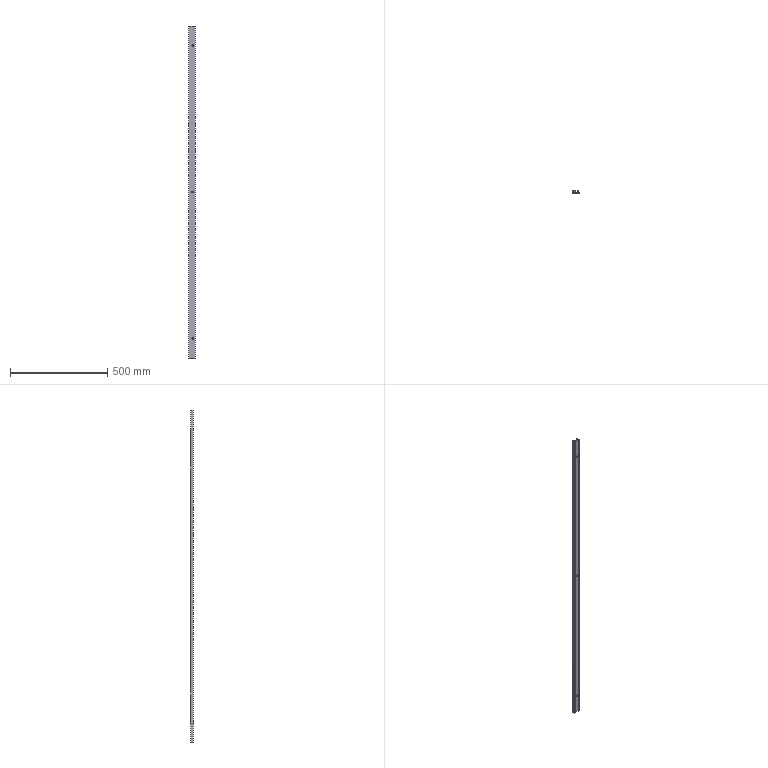Part | SolidWorks | features BaseBody 1, HoleWzd 1, ICE 1, MoveFace 1 | 1 solid | 31 faces | box 33.5 x 13.5 x 1705 mm | volume 319217 mm3 | plane 16 | cylinder 9 | cone 6 | commonest cylinder face diameters 2 x3 13.44 x3 4 x2 1.5 x1
STEP:
#1=CARTESIAN_POINT('',(20.,0.,1508.72));
#2=VERTEX_POINT('',#1);
#3=CARTESIAN_POINT('',(20.,0.,1501.28));
#4=VERTEX_POINT('',#3);
#5=CARTESIAN_POINT('',(20.,0.,1505.));
#6=DIRECTION('',(0.,-1.,0.));
#7=DIRECTION('',(0.,0.,-1.));
#8=AXIS2_PLACEMENT_3D('',#5,#6,#7);
#9=CIRCLE('',#8,3.72);
#10=EDGE_CURVE('',#2,#4,#9,.T.);
#11=ORIENTED_EDGE('',*,*,#10,.T.);
#12=CARTESIAN_POINT('',(20.,3.,1498.28));
#13=VERTEX_POINT('',#12);
#14=CARTESIAN_POINT('',(20.,3.,1498.28));
#15=DIRECTION('',(0.,0.7071,-0.7071));
#16=VECTOR('',#15,1000.);
#17=LINE('',#14,#16);
#18=EDGE_CURVE('',#4,#13,#17,.T.);
#19=ORIENTED_EDGE('',*,*,#18,.T.);
#20=CARTESIAN_POINT('',(20.,3.,1511.72));
#21=VERTEX_POINT('',#20);
#22=CARTESIAN_POINT('',(20.,3.,1505.));
#23=DIRECTION('',(0.,1.,0.));
#24=DIRECTION('',(0.,0.,1.));
#25=AXIS2_PLACEMENT_3D('',#22,#23,#24);
#26=CIRCLE('',#25,6.72);
#27=EDGE_CURVE('',#13,#21,#26,.T.);
#28=ORIENTED_EDGE('',*,*,#27,.T.);
#29=CARTESIAN_POINT('',(20.,3.,1511.72));
#30=DIRECTION('',(0.,0.7071,0.7071));
#31=VECTOR('',#30,1000.);
#32=LINE('',#29,#31);
#33=EDGE_CURVE('',#2,#21,#32,.T.);
#34=ORIENTED_EDGE('',*,*,#33,.F.);
#35=EDGE_LOOP('',(#11,#19,#28,#34));
#36=FACE_OUTER_BOUND('',#35,.T.);
#37=CARTESIAN_POINT('',(20.,3.,1505.));
#38=DIRECTION('',(0.,1.,0.));
#39=DIRECTION('',(0.,0.,1.));
#40=AXIS2_PLACEMENT_3D('',#37,#38,#39);
#41=CONICAL_SURFACE('',#40,6.72,0.7854);
#42=ADVANCED_FACE('',(#36),#41,.F.);
#43=CARTESIAN_POINT('',(20.,0.,3.72));
#44=VERTEX_POINT('',#43);
#45=CARTESIAN_POINT('',(20.,0.,-3.72));
#46=VERTEX_POINT('',#45);
#47=CARTESIAN_POINT('',(20.,0.,0.));
#48=DIRECTION('',(0.,-1.,0.));
#49=DIRECTION('',(0.,0.,-1.));
#50=AXIS2_PLACEMENT_3D('',#47,#48,#49);
#51=CIRCLE('',#50,3.72);
#52=EDGE_CURVE('',#44,#46,#51,.T.);
#53=ORIENTED_EDGE('',*,*,#52,.T.);
#54=CARTESIAN_POINT('',(20.,3.,-6.72));
#55=VERTEX_POINT('',#54);
#56=CARTESIAN_POINT('',(20.,3.,-6.72));
#57=DIRECTION('',(0.,0.7071,-0.7071));
#58=VECTOR('',#57,1000.);
#59=LINE('',#56,#58);
#60=EDGE_CURVE('',#46,#55,#59,.T.);
#61=ORIENTED_EDGE('',*,*,#60,.T.);
#62=CARTESIAN_POINT('',(20.,3.,6.72));
#63=VERTEX_POINT('',#62);
#64=CARTESIAN_POINT('',(20.,3.,0.));
#65=DIRECTION('',(0.,1.,0.));
#66=DIRECTION('',(0.,0.,1.));
#67=AXIS2_PLACEMENT_3D('',#64,#65,#66);
#68=CIRCLE('',#67,6.72);
#69=EDGE_CURVE('',#55,#63,#68,.T.);
#70=ORIENTED_EDGE('',*,*,#69,.T.);
#71=CARTESIAN_POINT('',(20.,3.,6.72));
#72=DIRECTION('',(0.,0.7071,0.7071));
#73=VECTOR('',#72,1000.);
#74=LINE('',#71,#73);
#75=EDGE_CURVE('',#44,#63,#74,.T.);
#76=ORIENTED_EDGE('',*,*,#75,.F.);
#77=EDGE_LOOP('',(#53,#61,#70,#76));
#78=FACE_OUTER_BOUND('',#77,.T.);
#79=CARTESIAN_POINT('',(20.,3.,0.));
#80=DIRECTION('',(0.,1.,0.));
#81=DIRECTION('',(0.,0.,1.));
#82=AXIS2_PLACEMENT_3D('',#79,#80,#81);
#83=CONICAL_SURFACE('',#82,6.72,0.7854);
#84=ADVANCED_FACE('',(#78),#83,.F.);
#85=CARTESIAN_POINT('',(20.,0.,756.22));
#86=VERTEX_POINT('',#85);
#87=CARTESIAN_POINT('',(20.,0.,748.78));
#88=VERTEX_POINT('',#87);
#89=CARTESIAN_POINT('',(20.,0.,752.5));
#90=DIRECTION('',(0.,-1.,0.));
#91=DIRECTION('',(0.,0.,-1.));
#92=AXIS2_PLACEMENT_3D('',#89,#90,#91);
#93=CIRCLE('',#92,3.72);
#94=EDGE_CURVE('',#86,#88,#93,.T.);
#95=ORIENTED_EDGE('',*,*,#94,.T.);
#96=CARTESIAN_POINT('',(20.,3.,745.78));
#97=VERTEX_POINT('',#96);
#98=CARTESIAN_POINT('',(20.,3.,745.78));
#99=DIRECTION('',(0.,0.7071,-0.7071));
#100=VECTOR('',#99,1000.);
#101=LINE('',#98,#100);
#102=EDGE_CURVE('',#88,#97,#101,.T.);
#103=ORIENTED_EDGE('',*,*,#102,.T.);
#104=CARTESIAN_POINT('',(20.,3.,759.22));
#105=VERTEX_POINT('',#104);
#106=CARTESIAN_POINT('',(20.,3.,752.5));
#107=DIRECTION('',(0.,1.,0.));
#108=DIRECTION('',(0.,0.,1.));
#109=AXIS2_PLACEMENT_3D('',#106,#107,#108);
#110=CIRCLE('',#109,6.72);
#111=EDGE_CURVE('',#97,#105,#110,.T.);
#112=ORIENTED_EDGE('',*,*,#111,.T.);
#113=CARTESIAN_POINT('',(20.,3.,759.22));
#114=DIRECTION('',(0.,0.7071,0.7071));
#115=VECTOR('',#114,1000.);
#116=LINE('',#113,#115);
#117=EDGE_CURVE('',#86,#105,#116,.T.);
#118=ORIENTED_EDGE('',*,*,#117,.F.);
#119=EDGE_LOOP('',(#95,#103,#112,#118));
#120=FACE_OUTER_BOUND('',#119,.T.);
#121=CARTESIAN_POINT('',(20.,3.,752.5));
#122=DIRECTION('',(0.,1.,0.));
#123=DIRECTION('',(0.,0.,1.));
#124=AXIS2_PLACEMENT_3D('',#121,#122,#123);
#125=CONICAL_SURFACE('',#124,6.72,0.7854);
#126=ADVANCED_FACE('',(#120),#125,.F.);
#127=CARTESIAN_POINT('',(24.5,10.5,-4.991));
#128=VERTEX_POINT('',#127);
#129=CARTESIAN_POINT('',(24.5,10.5,-100.));
#130=VERTEX_POINT('',#129);
#131=CARTESIAN_POINT('',(24.5,10.5,-100.));
#132=DIRECTION('',(0.,0.,-1.));
#133=VECTOR('',#132,1000.);
#134=LINE('',#131,#133);
#135=EDGE_CURVE('',#128,#130,#134,.T.);
#136=ORIENTED_EDGE('',*,*,#135,.F.);
#137=CARTESIAN_POINT('',(24.5,10.5,4.991));
#138=VERTEX_POINT('',#137);
#139=CARTESIAN_POINT('',(24.5,10.5,-4.991));
#140=CARTESIAN_POINT('',(24.5,10.638,-4.991));
#141=CARTESIAN_POINT('',(24.515,10.777,-4.978));
#142=CARTESIAN_POINT('',(24.57,11.043,-4.927));
#143=CARTESIAN_POINT('',(24.611,11.171,-4.889));
#144=CARTESIAN_POINT('',(24.765,11.529,-4.74));
#145=CARTESIAN_POINT('',(24.907,11.728,-4.597));
#146=CARTESIAN_POINT('',(25.205,12.04,-4.256));
#147=CARTESIAN_POINT('',(25.365,12.156,-4.055));
#148=CARTESIAN_POINT('',(25.663,12.325,-3.627));
#149=CARTESIAN_POINT('',(25.806,12.38,-3.395));
#150=CARTESIAN_POINT('',(26.19,12.494,-2.672));
#151=CARTESIAN_POINT('',(26.387,12.501,-2.161));
#152=CARTESIAN_POINT('',(26.654,12.499,-1.091));
#153=CARTESIAN_POINT('',(26.72,12.488,-0.5481));
#154=CARTESIAN_POINT('',(26.72,12.488,0.2773));
#155=CARTESIAN_POINT('',(26.703,12.49,0.5529));
#156=CARTESIAN_POINT('',(26.636,12.496,1.095));
#157=CARTESIAN_POINT('',(26.586,12.499,1.362));
#158=CARTESIAN_POINT('',(26.388,12.501,2.155));
#159=CARTESIAN_POINT('',(26.188,12.493,2.677));
#160=CARTESIAN_POINT('',(25.805,12.38,3.396));
#161=CARTESIAN_POINT('',(25.662,12.324,3.629));
#162=CARTESIAN_POINT('',(25.438,12.197,3.95));
#163=CARTESIAN_POINT('',(25.362,12.147,4.053));
#164=CARTESIAN_POINT('',(25.208,12.03,4.249));
#165=CARTESIAN_POINT('',(25.13,11.961,4.342));
#166=CARTESIAN_POINT('',(24.98,11.805,4.513));
#167=CARTESIAN_POINT('',(24.908,11.717,4.591));
#168=CARTESIAN_POINT('',(24.774,11.518,4.73));
#169=CARTESIAN_POINT('',(24.714,11.408,4.79));
#170=CARTESIAN_POINT('',(24.612,11.172,4.888));
#171=CARTESIAN_POINT('',(24.57,11.043,4.927));
#172=CARTESIAN_POINT('',(24.515,10.778,4.978));
#173=CARTESIAN_POINT('',(24.5,10.64,4.991));
#174=CARTESIAN_POINT('',(24.5,10.5,4.991));
#175=B_SPLINE_CURVE_WITH_KNOTS('',3,(#139,#140,#141,#142,#143,#144,#145,#146,#147,#148,#149,#150,#151,#152,#153,#154,#155,#156,#157,#158,#159,#160,#161,#162,#163,#164,#165,#166,#167,#168,#169,#170,#171,#172,#173,#174),.UNSPECIFIED.,.F.,.F.,(4,2,2,2,2,2,2,2,2,2,2,2,2,2,2,2,2,4),(0.01321,0.01362,0.01403,0.01486,0.01569,0.01651,0.01816,0.01981,0.02064,0.02146,0.02311,0.02394,0.02435,0.02477,0.02518,0.02559,0.026,0.02642),.UNSPECIFIED.);
#176=EDGE_CURVE('',#128,#138,#175,.T.);
#177=ORIENTED_EDGE('',*,*,#176,.T.);
#178=CARTESIAN_POINT('',(24.5,10.5,747.509));
#179=VERTEX_POINT('',#178);
#180=CARTESIAN_POINT('',(24.5,10.5,-100.));
#181=DIRECTION('',(0.,0.,-1.));
#182=VECTOR('',#181,1000.);
#183=LINE('',#180,#182);
#184=EDGE_CURVE('',#179,#138,#183,.T.);
#185=ORIENTED_EDGE('',*,*,#184,.F.);
#186=CARTESIAN_POINT('',(24.5,10.5,757.491));
#187=VERTEX_POINT('',#186);
#188=CARTESIAN_POINT('',(24.5,10.5,747.509));
#189=CARTESIAN_POINT('',(24.5,10.638,747.509));
#190=CARTESIAN_POINT('',(24.515,10.777,747.522));
#191=CARTESIAN_POINT('',(24.57,11.043,747.573));
#192=CARTESIAN_POINT('',(24.611,11.171,747.611));
#193=CARTESIAN_POINT('',(24.765,11.529,747.76));
#194=CARTESIAN_POINT('',(24.907,11.728,747.903));
#195=CARTESIAN_POINT('',(25.205,12.04,748.244));
#196=CARTESIAN_POINT('',(25.365,12.156,748.445));
#197=CARTESIAN_POINT('',(25.663,12.325,748.873));
#198=CARTESIAN_POINT('',(25.806,12.38,749.105));
#199=CARTESIAN_POINT('',(26.19,12.494,749.828));
#200=CARTESIAN_POINT('',(26.387,12.501,750.339));
#201=CARTESIAN_POINT('',(26.654,12.499,751.409));
#202=CARTESIAN_POINT('',(26.72,12.488,751.952));
#203=CARTESIAN_POINT('',(26.72,12.488,752.777));
#204=CARTESIAN_POINT('',(26.703,12.49,753.053));
#205=CARTESIAN_POINT('',(26.636,12.496,753.595));
#206=CARTESIAN_POINT('',(26.586,12.499,753.862));
#207=CARTESIAN_POINT('',(26.388,12.501,754.655));
#208=CARTESIAN_POINT('',(26.188,12.493,755.177));
#209=CARTESIAN_POINT('',(25.805,12.38,755.896));
#210=CARTESIAN_POINT('',(25.662,12.324,756.129));
#211=CARTESIAN_POINT('',(25.438,12.197,756.45));
#212=CARTESIAN_POINT('',(25.362,12.147,756.553));
#213=CARTESIAN_POINT('',(25.208,12.03,756.749));
#214=CARTESIAN_POINT('',(25.13,11.961,756.842));
#215=CARTESIAN_POINT('',(24.98,11.805,757.013));
#216=CARTESIAN_POINT('',(24.908,11.717,757.091));
#217=CARTESIAN_POINT('',(24.774,11.518,757.23));
#218=CARTESIAN_POINT('',(24.714,11.408,757.29));
#219=CARTESIAN_POINT('',(24.612,11.172,757.388));
#220=CARTESIAN_POINT('',(24.57,11.043,757.427));
#221=CARTESIAN_POINT('',(24.515,10.778,757.478));
#222=CARTESIAN_POINT('',(24.5,10.64,757.491));
#223=CARTESIAN_POINT('',(24.5,10.5,757.491));
#224=B_SPLINE_CURVE_WITH_KNOTS('',3,(#188,#189,#190,#191,#192,#193,#194,#195,#196,#197,#198,#199,#200,#201,#202,#203,#204,#205,#206,#207,#208,#209,#210,#211,#212,#213,#214,#215,#216,#217,#218,#219,#220,#221,#222,#223),.UNSPECIFIED.,.F.,.F.,(4,2,2,2,2,2,2,2,2,2,2,2,2,2,2,2,2,4),(0.01321,0.01362,0.01403,0.01486,0.01569,0.01651,0.01816,0.01981,0.02064,0.02146,0.02311,0.02394,0.02435,0.02477,0.02518,0.02559,0.026,0.02642),.UNSPECIFIED.);
#225=EDGE_CURVE('',#179,#187,#224,.T.);
#226=ORIENTED_EDGE('',*,*,#225,.T.);
#227=CARTESIAN_POINT('',(24.5,10.5,1500.009));
#228=VERTEX_POINT('',#227);
#229=CARTESIAN_POINT('',(24.5,10.5,-100.));
#230=DIRECTION('',(0.,0.,-1.));
#231=VECTOR('',#230,1000.);
#232=LINE('',#229,#231);
#233=EDGE_CURVE('',#228,#187,#232,.T.);
#234=ORIENTED_EDGE('',*,*,#233,.F.);
#235=CARTESIAN_POINT('',(24.5,10.5,1509.991));
#236=VERTEX_POINT('',#235);
#237=CARTESIAN_POINT('',(24.5,10.5,1500.009));
#238=CARTESIAN_POINT('',(24.5,10.64,1500.009));
#239=CARTESIAN_POINT('',(24.514,10.776,1500.022));
#240=CARTESIAN_POINT('',(24.57,11.042,1500.073));
#241=CARTESIAN_POINT('',(24.611,11.171,1500.111));
#242=CARTESIAN_POINT('',(24.713,11.408,1500.209));
#243=CARTESIAN_POINT('',(24.775,11.519,1500.27));
#244=CARTESIAN_POINT('',(24.908,11.717,1500.409));
#245=CARTESIAN_POINT('',(24.981,11.806,1500.488));
#246=CARTESIAN_POINT('',(25.207,12.042,1500.746));
#247=CARTESIAN_POINT('',(25.363,12.155,1500.942));
#248=CARTESIAN_POINT('',(25.665,12.326,1501.376));
#249=CARTESIAN_POINT('',(25.806,12.38,1501.605));
#250=CARTESIAN_POINT('',(26.061,12.456,1502.084));
#251=CARTESIAN_POINT('',(26.176,12.476,1502.337));
#252=CARTESIAN_POINT('',(26.372,12.498,1502.849));
#253=CARTESIAN_POINT('',(26.454,12.501,1503.109));
#254=CARTESIAN_POINT('',(26.586,12.499,1503.638));
#255=CARTESIAN_POINT('',(26.636,12.496,1503.907));
#256=CARTESIAN_POINT('',(26.703,12.49,1504.453));
#257=CARTESIAN_POINT('',(26.72,12.488,1504.729));
#258=CARTESIAN_POINT('',(26.72,12.488,1505.275));
#259=CARTESIAN_POINT('',(26.703,12.49,1505.547));
#260=CARTESIAN_POINT('',(26.637,12.496,1506.089));
#261=CARTESIAN_POINT('',(26.587,12.499,1506.36));
#262=CARTESIAN_POINT('',(26.387,12.501,1507.161));
#263=CARTESIAN_POINT('',(26.191,12.494,1507.671));
#264=CARTESIAN_POINT('',(25.805,12.38,1508.396));
#265=CARTESIAN_POINT('',(25.663,12.325,1508.627));
#266=CARTESIAN_POINT('',(25.364,12.155,1509.057));
#267=CARTESIAN_POINT('',(25.205,12.039,1509.256));
#268=CARTESIAN_POINT('',(24.981,11.805,1509.512));
#269=CARTESIAN_POINT('',(24.907,11.716,1509.592));
#270=CARTESIAN_POINT('',(24.774,11.518,1509.73));
#271=CARTESIAN_POINT('',(24.714,11.409,1509.79));
#272=CARTESIAN_POINT('',(24.611,11.17,1509.889));
#273=CARTESIAN_POINT('',(24.571,11.044,1509.926));
#274=CARTESIAN_POINT('',(24.515,10.78,1509.977));
#275=CARTESIAN_POINT('',(24.5,10.64,1509.991));
#276=CARTESIAN_POINT('',(24.5,10.5,1509.991));
#277=B_SPLINE_CURVE_WITH_KNOTS('',3,(#237,#238,#239,#240,#241,#242,#243,#244,#245,#246,#247,#248,#249,#250,#251,#252,#253,#254,#255,#256,#257,#258,#259,#260,#261,#262,#263,#264,#265,#266,#267,#268,#269,#270,#271,#272,#273,#274,#275,#276),.UNSPECIFIED.,.F.,.F.,(4,2,2,2,2,2,2,2,2,2,2,2,2,2,2,2,2,2,2,4),(0.,0.0004127,0.0008255,0.001238,0.001651,0.002476,0.003302,0.004127,0.004953,0.005778,0.006604,0.007429,0.008255,0.009906,0.01073,0.01156,0.01197,0.01238,0.01279,0.01321),.UNSPECIFIED.);
#278=EDGE_CURVE('',#228,#236,#277,.T.);
#279=ORIENTED_EDGE('',*,*,#278,.T.);
#280=CARTESIAN_POINT('',(24.5,10.5,1605.));
#281=VERTEX_POINT('',#280);
#282=CARTESIAN_POINT('',(24.5,10.5,-100.));
#283=DIRECTION('',(0.,0.,-1.));
#284=VECTOR('',#283,1000.);
#285=LINE('',#282,#284);
#286=EDGE_CURVE('',#281,#236,#285,.T.);
#287=ORIENTED_EDGE('',*,*,#286,.F.);
#288=CARTESIAN_POINT('',(28.5,10.5,1605.));
#289=VERTEX_POINT('',#288);
#290=CARTESIAN_POINT('',(26.5,10.5,1605.));
#291=DIRECTION('',(0.,0.,1.));
#292=DIRECTION('',(1.,0.,0.));
#293=AXIS2_PLACEMENT_3D('',#290,#291,#292);
#294=CIRCLE('',#293,2.);
#295=EDGE_CURVE('',#289,#281,#294,.T.);
#296=ORIENTED_EDGE('',*,*,#295,.F.);
#297=CARTESIAN_POINT('',(28.5,10.5,-100.));
#298=VERTEX_POINT('',#297);
#299=CARTESIAN_POINT('',(28.5,10.5,-100.));
#300=DIRECTION('',(0.,0.,-1.));
#301=VECTOR('',#300,1000.);
#302=LINE('',#299,#301);
#303=EDGE_CURVE('',#289,#298,#302,.T.);
#304=ORIENTED_EDGE('',*,*,#303,.T.);
#305=CARTESIAN_POINT('',(26.5,10.5,-100.));
#306=DIRECTION('',(0.,0.,1.));
#307=DIRECTION('',(-1.,0.,0.));
#308=AXIS2_PLACEMENT_3D('',#305,#306,#307);
#309=CIRCLE('',#308,2.);
#310=EDGE_CURVE('',#298,#130,#309,.T.);
#311=ORIENTED_EDGE('',*,*,#310,.T.);
#312=EDGE_LOOP('',(#136,#177,#185,#226,#234,#279,#287,#296,#304,#311));
#313=FACE_OUTER_BOUND('',#312,.T.);
#314=CARTESIAN_POINT('',(26.5,10.5,-100.));
#315=DIRECTION('',(0.,0.,-1.));
#316=DIRECTION('',(-1.,0.,0.));
#317=AXIS2_PLACEMENT_3D('',#314,#315,#316);
#318=CYLINDRICAL_SURFACE('',#317,2.);
#319=ADVANCED_FACE('',(#313),#318,.T.);
#320=CARTESIAN_POINT('',(24.5,3.,-4.991));
#321=VERTEX_POINT('',#320);
#322=CARTESIAN_POINT('',(24.5,3.,-100.));
#323=VERTEX_POINT('',#322);
#324=CARTESIAN_POINT('',(24.5,3.,-100.));
#325=DIRECTION('',(0.,0.,-1.));
#326=VECTOR('',#325,1000.);
#327=LINE('',#324,#326);
#328=EDGE_CURVE('',#321,#323,#327,.T.);
#329=ORIENTED_EDGE('',*,*,#328,.F.);
#330=CARTESIAN_POINT('',(24.5,13.5,-4.991));
#331=DIRECTION('',(0.,1.,0.));
#332=VECTOR('',#331,1000.);
#333=LINE('',#330,#332);
#334=EDGE_CURVE('',#321,#128,#333,.T.);
#335=ORIENTED_EDGE('',*,*,#334,.T.);
#336=ORIENTED_EDGE('',*,*,#135,.T.);
#337=CARTESIAN_POINT('',(24.5,1.,-100.));
#338=DIRECTION('',(0.,-1.,0.));
#339=VECTOR('',#338,1000.);
#340=LINE('',#337,#339);
#341=EDGE_CURVE('',#130,#323,#340,.T.);
#342=ORIENTED_EDGE('',*,*,#341,.T.);
#343=EDGE_LOOP('',(#329,#335,#336,#342));
#344=FACE_OUTER_BOUND('',#343,.T.);
#345=CARTESIAN_POINT('',(24.5,10.5,-100.));
#346=DIRECTION('',(-1.,0.,0.));
#347=DIRECTION('',(0.,0.,1.));
#348=AXIS2_PLACEMENT_3D('',#345,#346,#347);
#349=PLANE('',#348);
#350=ADVANCED_FACE('',(#344),#349,.T.);
#351=ORIENTED_EDGE('',*,*,#184,.T.);
#352=CARTESIAN_POINT('',(24.5,3.,4.991));
#353=VERTEX_POINT('',#352);
#354=CARTESIAN_POINT('',(24.5,13.5,4.991));
#355=DIRECTION('',(0.,-1.,0.));
#356=VECTOR('',#355,1000.);
#357=LINE('',#354,#356);
#358=EDGE_CURVE('',#138,#353,#357,.T.);
#359=ORIENTED_EDGE('',*,*,#358,.T.);
#360=CARTESIAN_POINT('',(24.5,3.,747.509));
#361=VERTEX_POINT('',#360);
#362=CARTESIAN_POINT('',(24.5,3.,-100.));
#363=DIRECTION('',(0.,0.,-1.));
#364=VECTOR('',#363,1000.);
#365=LINE('',#362,#364);
#366=EDGE_CURVE('',#361,#353,#365,.T.);
#367=ORIENTED_EDGE('',*,*,#366,.F.);
#368=CARTESIAN_POINT('',(24.5,13.5,747.509));
#369=DIRECTION('',(0.,1.,0.));
#370=VECTOR('',#369,1000.);
#371=LINE('',#368,#370);
#372=EDGE_CURVE('',#361,#179,#371,.T.);
#373=ORIENTED_EDGE('',*,*,#372,.T.);
#374=EDGE_LOOP('',(#351,#359,#367,#373));
#375=FACE_OUTER_BOUND('',#374,.T.);
#376=CARTESIAN_POINT('',(24.5,10.5,-100.));
#377=DIRECTION('',(-1.,0.,0.));
#378=DIRECTION('',(0.,0.,1.));
#379=AXIS2_PLACEMENT_3D('',#376,#377,#378);
#380=PLANE('',#379);
#381=ADVANCED_FACE('',(#375),#380,.T.);
#382=ORIENTED_EDGE('',*,*,#233,.T.);
#383=CARTESIAN_POINT('',(24.5,3.,757.491));
#384=VERTEX_POINT('',#383);
#385=CARTESIAN_POINT('',(24.5,13.5,757.491));
#386=DIRECTION('',(0.,-1.,0.));
#387=VECTOR('',#386,1000.);
#388=LINE('',#385,#387);
#389=EDGE_CURVE('',#187,#384,#388,.T.);
#390=ORIENTED_EDGE('',*,*,#389,.T.);
#391=CARTESIAN_POINT('',(24.5,3.,1500.009));
#392=VERTEX_POINT('',#391);
#393=CARTESIAN_POINT('',(24.5,3.,-100.));
#394=DIRECTION('',(0.,0.,-1.));
#395=VECTOR('',#394,1000.);
#396=LINE('',#393,#395);
#397=EDGE_CURVE('',#392,#384,#396,.T.);
#398=ORIENTED_EDGE('',*,*,#397,.F.);
#399=CARTESIAN_POINT('',(24.5,13.5,1500.009));
#400=DIRECTION('',(0.,1.,0.));
#401=VECTOR('',#400,1000.);
#402=LINE('',#399,#401);
#403=EDGE_CURVE('',#392,#228,#402,.T.);
#404=ORIENTED_EDGE('',*,*,#403,.T.);
#405=EDGE_LOOP('',(#382,#390,#398,#404));
#406=FACE_OUTER_BOUND('',#405,.T.);
#407=CARTESIAN_POINT('',(24.5,10.5,-100.));
#408=DIRECTION('',(-1.,0.,0.));
#409=DIRECTION('',(0.,0.,1.));
#410=AXIS2_PLACEMENT_3D('',#407,#408,#409);
#411=PLANE('',#410);
#412=ADVANCED_FACE('',(#406),#411,.T.);
#413=ORIENTED_EDGE('',*,*,#286,.T.);
#414=CARTESIAN_POINT('',(24.5,3.,1509.991));
#415=VERTEX_POINT('',#414);
#416=CARTESIAN_POINT('',(24.5,13.5,1509.991));
#417=DIRECTION('',(0.,-1.,0.));
#418=VECTOR('',#417,1000.);
#419=LINE('',#416,#418);
#420=EDGE_CURVE('',#236,#415,#419,.T.);
#421=ORIENTED_EDGE('',*,*,#420,.T.);
#422=CARTESIAN_POINT('',(24.5,3.,1605.));
#423=VERTEX_POINT('',#422);
#424=CARTESIAN_POINT('',(24.5,3.,-100.));
#425=DIRECTION('',(0.,0.,-1.));
#426=VECTOR('',#425,1000.);
#427=LINE('',#424,#426);
#428=EDGE_CURVE('',#423,#415,#427,.T.);
#429=ORIENTED_EDGE('',*,*,#428,.F.);
#430=CARTESIAN_POINT('',(24.5,1.,1605.));
#431=DIRECTION('',(0.,-1.,0.));
#432=VECTOR('',#431,1000.);
#433=LINE('',#430,#432);
#434=EDGE_CURVE('',#281,#423,#433,.T.);
#435=ORIENTED_EDGE('',*,*,#434,.F.);
#436=EDGE_LOOP('',(#413,#421,#429,#435));
#437=FACE_OUTER_BOUND('',#436,.T.);
#438=CARTESIAN_POINT('',(24.5,10.5,-100.));
#439=DIRECTION('',(-1.,0.,0.));
#440=DIRECTION('',(0.,0.,1.));
#441=AXIS2_PLACEMENT_3D('',#438,#439,#440);
#442=PLANE('',#441);
#443=ADVANCED_FACE('',(#437),#442,.T.);
#444=ORIENTED_EDGE('',*,*,#10,.F.);
#445=CARTESIAN_POINT('',(20.,0.,1505.));
#446=DIRECTION('',(0.,-1.,0.));
#447=DIRECTION('',(0.,0.,-1.));
#448=AXIS2_PLACEMENT_3D('',#445,#446,#447);
#449=CIRCLE('',#448,3.72);
#450=EDGE_CURVE('',#4,#2,#449,.T.);
#451=ORIENTED_EDGE('',*,*,#450,.F.);
#452=EDGE_LOOP('',(#444,#451));
#453=FACE_BOUND('',#452,.T.);
#454=ORIENTED_EDGE('',*,*,#94,.F.);
#455=CARTESIAN_POINT('',(20.,0.,752.5));
#456=DIRECTION('',(0.,-1.,0.));
#457=DIRECTION('',(0.,0.,-1.));
#458=AXIS2_PLACEMENT_3D('',#455,#456,#457);
#459=CIRCLE('',#458,3.72);
#460=EDGE_CURVE('',#88,#86,#459,.T.);
#461=ORIENTED_EDGE('',*,*,#460,.F.);
#462=EDGE_LOOP('',(#454,#461));
#463=FACE_BOUND('',#462,.T.);
#464=CARTESIAN_POINT('',(1.,0.,-100.));
#465=VERTEX_POINT('',#464);
#466=CARTESIAN_POINT('',(32.5,0.,-100.));
#467=VERTEX_POINT('',#466);
#468=CARTESIAN_POINT('',(1.,0.,-100.));
#469=DIRECTION('',(1.,0.,0.));
#470=VECTOR('',#469,1000.);
#471=LINE('',#468,#470);
#472=EDGE_CURVE('',#465,#467,#471,.T.);
#473=ORIENTED_EDGE('',*,*,#472,.T.);
#474=CARTESIAN_POINT('',(32.5,0.,1605.));
#475=VERTEX_POINT('',#474);
#476=CARTESIAN_POINT('',(32.5,0.,-100.));
#477=DIRECTION('',(0.,0.,1.));
#478=VECTOR('',#477,1000.);
#479=LINE('',#476,#478);
#480=EDGE_CURVE('',#467,#475,#479,.T.);
#481=ORIENTED_EDGE('',*,*,#480,.T.);
#482=CARTESIAN_POINT('',(1.,0.,1605.));
#483=VERTEX_POINT('',#482);
#484=CARTESIAN_POINT('',(1.,0.,1605.));
#485=DIRECTION('',(-1.,0.,0.));
#486=VECTOR('',#485,1000.);
#487=LINE('',#484,#486);
#488=EDGE_CURVE('',#475,#483,#487,.T.);
#489=ORIENTED_EDGE('',*,*,#488,.T.);
#490=CARTESIAN_POINT('',(1.,0.,-100.));
#491=DIRECTION('',(0.,0.,-1.));
#492=VECTOR('',#491,1000.);
#493=LINE('',#490,#492);
#494=EDGE_CURVE('',#483,#465,#493,.T.);
#495=ORIENTED_EDGE('',*,*,#494,.T.);
#496=EDGE_LOOP('',(#473,#481,#489,#495));
#497=FACE_OUTER_BOUND('',#496,.T.);
#498=ORIENTED_EDGE('',*,*,#52,.F.);
#499=CARTESIAN_POINT('',(20.,0.,0.));
#500=DIRECTION('',(0.,-1.,0.));
#501=DIRECTION('',(0.,0.,-1.));
#502=AXIS2_PLACEMENT_3D('',#499,#500,#501);
#503=CIRCLE('',#502,3.72);
#504=EDGE_CURVE('',#46,#44,#503,.T.);
#505=ORIENTED_EDGE('',*,*,#504,.F.);
#506=EDGE_LOOP('',(#498,#505));
#507=FACE_BOUND('',#506,.T.);
#508=CARTESIAN_POINT('',(1.,0.,-100.));
#509=DIRECTION('',(0.,-1.,0.));
#510=DIRECTION('',(0.,0.,-1.));
#511=AXIS2_PLACEMENT_3D('',#508,#509,#510);
#512=PLANE('',#511);
#513=ADVANCED_FACE('',(#453,#463,#497,#507),#512,.T.);
#514=CARTESIAN_POINT('',(33.5,1.,-100.));
#515=VERTEX_POINT('',#514);
#516=CARTESIAN_POINT('',(32.5,1.,-100.));
#517=DIRECTION('',(0.,0.,1.));
#518=DIRECTION('',(-1.,0.,0.));
#519=AXIS2_PLACEMENT_3D('',#516,#517,#518);
#520=CIRCLE('',#519,1.);
#521=EDGE_CURVE('',#467,#515,#520,.T.);
#522=ORIENTED_EDGE('',*,*,#521,.T.);
#523=CARTESIAN_POINT('',(33.5,1.,1605.));
#524=VERTEX_POINT('',#523);
#525=CARTESIAN_POINT('',(33.5,1.,-100.));
#526=DIRECTION('',(0.,0.,1.));
#527=VECTOR('',#526,1000.);
#528=LINE('',#525,#527);
#529=EDGE_CURVE('',#515,#524,#528,.T.);
#530=ORIENTED_EDGE('',*,*,#529,.T.);
#531=CARTESIAN_POINT('',(32.5,1.,1605.));
#532=DIRECTION('',(0.,0.,-1.));
#533=DIRECTION('',(1.,0.,0.));
#534=AXIS2_PLACEMENT_3D('',#531,#532,#533);
#535=CIRCLE('',#534,1.);
#536=EDGE_CURVE('',#524,#475,#535,.T.);
#537=ORIENTED_EDGE('',*,*,#536,.T.);
#538=ORIENTED_EDGE('',*,*,#480,.F.);
#539=EDGE_LOOP('',(#522,#530,#537,#538));
#540=FACE_OUTER_BOUND('',#539,.T.);
#541=CARTESIAN_POINT('',(32.5,1.,-100.));
#542=DIRECTION('',(0.,0.,-1.));
#543=DIRECTION('',(-1.,0.,0.));
#544=AXIS2_PLACEMENT_3D('',#541,#542,#543);
#545=CYLINDRICAL_SURFACE('',#544,1.);
#546=ADVANCED_FACE('',(#540),#545,.T.);
#547=CARTESIAN_POINT('',(1.5,12.75,-100.));
#548=VERTEX_POINT('',#547);
#549=CARTESIAN_POINT('',(0.,12.75,-100.));
#550=VERTEX_POINT('',#549);
#551=CARTESIAN_POINT('',(0.75,12.75,-100.));
#552=DIRECTION('',(0.,0.,1.));
#553=DIRECTION('',(-1.,0.,0.));
#554=AXIS2_PLACEMENT_3D('',#551,#552,#553);
#555=CIRCLE('',#554,0.75);
#556=EDGE_CURVE('',#548,#550,#555,.T.);
#557=ORIENTED_EDGE('',*,*,#556,.F.);
#558=CARTESIAN_POINT('',(1.5,3.,-100.));
#559=VERTEX_POINT('',#558);
#560=CARTESIAN_POINT('',(1.5,1.,-100.));
#561=DIRECTION('',(0.,1.,0.));
#562=VECTOR('',#561,1000.);
#563=LINE('',#560,#562);
#564=EDGE_CURVE('',#559,#548,#563,.T.);
#565=ORIENTED_EDGE('',*,*,#564,.F.);
#566=CARTESIAN_POINT('',(8.5,3.,-100.));
#567=VERTEX_POINT('',#566);
#568=CARTESIAN_POINT('',(1.,3.,-100.));
#569=DIRECTION('',(-1.,0.,0.));
#570=VECTOR('',#569,1000.);
#571=LINE('',#568,#570);
#572=EDGE_CURVE('',#567,#559,#571,.T.);
#573=ORIENTED_EDGE('',*,*,#572,.F.);
#574=CARTESIAN_POINT('',(8.5,10.5,-100.));
#575=VERTEX_POINT('',#574);
#576=CARTESIAN_POINT('',(8.5,1.,-100.));
#577=DIRECTION('',(0.,-1.,0.));
#578=VECTOR('',#577,1000.);
#579=LINE('',#576,#578);
#580=EDGE_CURVE('',#575,#567,#579,.T.);
#581=ORIENTED_EDGE('',*,*,#580,.F.);
#582=CARTESIAN_POINT('',(12.5,10.5,-100.));
#583=VERTEX_POINT('',#582);
#584=CARTESIAN_POINT('',(10.5,10.5,-100.));
#585=DIRECTION('',(0.,0.,1.));
#586=DIRECTION('',(-1.,0.,0.));
#587=AXIS2_PLACEMENT_3D('',#584,#585,#586);
#588=CIRCLE('',#587,2.);
#589=EDGE_CURVE('',#583,#575,#588,.T.);
#590=ORIENTED_EDGE('',*,*,#589,.F.);
#591=CARTESIAN_POINT('',(12.5,3.,-100.));
#592=VERTEX_POINT('',#591);
#593=CARTESIAN_POINT('',(12.5,1.,-100.));
#594=DIRECTION('',(0.,1.,0.));
#595=VECTOR('',#594,1000.);
#596=LINE('',#593,#595);
#597=EDGE_CURVE('',#592,#583,#596,.T.);
#598=ORIENTED_EDGE('',*,*,#597,.F.);
#599=CARTESIAN_POINT('',(1.,3.,-100.));
#600=DIRECTION('',(-1.,0.,0.));
#601=VECTOR('',#600,1000.);
#602=LINE('',#599,#601);
#603=EDGE_CURVE('',#323,#592,#602,.T.);
#604=ORIENTED_EDGE('',*,*,#603,.F.);
#605=ORIENTED_EDGE('',*,*,#341,.F.);
#606=ORIENTED_EDGE('',*,*,#310,.F.);
#607=CARTESIAN_POINT('',(28.5,3.,-100.));
#608=VERTEX_POINT('',#607);
#609=CARTESIAN_POINT('',(28.5,1.,-100.));
#610=DIRECTION('',(0.,1.,0.));
#611=VECTOR('',#610,1000.);
#612=LINE('',#609,#611);
#613=EDGE_CURVE('',#608,#298,#612,.T.);
#614=ORIENTED_EDGE('',*,*,#613,.F.);
#615=CARTESIAN_POINT('',(32.5,3.,-100.));
#616=VERTEX_POINT('',#615);
#617=CARTESIAN_POINT('',(1.,3.,-100.));
#618=DIRECTION('',(-1.,0.,0.));
#619=VECTOR('',#618,1000.);
#620=LINE('',#617,#619);
#621=EDGE_CURVE('',#616,#608,#620,.T.);
#622=ORIENTED_EDGE('',*,*,#621,.F.);
#623=CARTESIAN_POINT('',(33.5,2.,-100.));
#624=VERTEX_POINT('',#623);
#625=CARTESIAN_POINT('',(32.5,2.,-100.));
#626=DIRECTION('',(0.,0.,1.));
#627=DIRECTION('',(-1.,0.,0.));
#628=AXIS2_PLACEMENT_3D('',#625,#626,#627);
#629=CIRCLE('',#628,1.);
#630=EDGE_CURVE('',#624,#616,#629,.T.);
#631=ORIENTED_EDGE('',*,*,#630,.F.);
#632=CARTESIAN_POINT('',(33.5,1.,-100.));
#633=DIRECTION('',(0.,1.,0.));
#634=VECTOR('',#633,1000.);
#635=LINE('',#632,#634);
#636=EDGE_CURVE('',#515,#624,#635,.T.);
#637=ORIENTED_EDGE('',*,*,#636,.F.);
#638=ORIENTED_EDGE('',*,*,#521,.F.);
#639=ORIENTED_EDGE('',*,*,#472,.F.);
#640=CARTESIAN_POINT('',(0.,1.,-100.));
#641=VERTEX_POINT('',#640);
#642=CARTESIAN_POINT('',(1.,1.,-100.));
#643=DIRECTION('',(0.,0.,1.));
#644=DIRECTION('',(-1.,0.,0.));
#645=AXIS2_PLACEMENT_3D('',#642,#643,#644);
#646=CIRCLE('',#645,1.);
#647=EDGE_CURVE('',#641,#465,#646,.T.);
#648=ORIENTED_EDGE('',*,*,#647,.F.);
#649=CARTESIAN_POINT('',(0.,1.,-100.));
#650=DIRECTION('',(0.,-1.,0.));
#651=VECTOR('',#650,1000.);
#652=LINE('',#649,#651);
#653=EDGE_CURVE('',#550,#641,#652,.T.);
#654=ORIENTED_EDGE('',*,*,#653,.F.);
#655=EDGE_LOOP('',(#557,#565,#573,#581,#590,#598,#604,#605,#606,#614,#622,#631,#637,#638,#639,#648,#654));
#656=FACE_OUTER_BOUND('',#655,.T.);
#657=CARTESIAN_POINT('',(1.,1.,-100.));
#658=DIRECTION('',(0.,0.,1.));
#659=DIRECTION('',(1.,0.,0.));
#660=AXIS2_PLACEMENT_3D('',#657,#658,#659);
#661=PLANE('',#660);
#662=ADVANCED_FACE('',(#656),#661,.F.);
#663=ORIENTED_EDGE('',*,*,#647,.T.);
#664=ORIENTED_EDGE('',*,*,#494,.F.);
#665=CARTESIAN_POINT('',(0.,1.,1605.));
#666=VERTEX_POINT('',#665);
#667=CARTESIAN_POINT('',(1.,1.,1605.));
#668=DIRECTION('',(0.,0.,-1.));
#669=DIRECTION('',(1.,0.,0.));
#670=AXIS2_PLACEMENT_3D('',#667,#668,#669);
#671=CIRCLE('',#670,1.);
#672=EDGE_CURVE('',#483,#666,#671,.T.);
#673=ORIENTED_EDGE('',*,*,#672,.T.);
#674=CARTESIAN_POINT('',(0.,1.,-100.));
#675=DIRECTION('',(0.,0.,-1.));
#676=VECTOR('',#675,1000.);
#677=LINE('',#674,#676);
#678=EDGE_CURVE('',#666,#641,#677,.T.);
#679=ORIENTED_EDGE('',*,*,#678,.T.);
#680=EDGE_LOOP('',(#663,#664,#673,#679));
#681=FACE_OUTER_BOUND('',#680,.T.);
#682=CARTESIAN_POINT('',(1.,1.,-100.));
#683=DIRECTION('',(0.,0.,-1.));
#684=DIRECTION('',(-1.,0.,0.));
#685=AXIS2_PLACEMENT_3D('',#682,#683,#684);
#686=CYLINDRICAL_SURFACE('',#685,1.);
#687=ADVANCED_FACE('',(#681),#686,.T.);
#688=CARTESIAN_POINT('',(1.5,3.,1605.));
#689=VERTEX_POINT('',#688);
#690=CARTESIAN_POINT('',(1.5,12.75,1605.));
#691=VERTEX_POINT('',#690);
#692=CARTESIAN_POINT('',(1.5,1.,1605.));
#693=DIRECTION('',(0.,1.,0.));
#694=VECTOR('',#693,1000.);
#695=LINE('',#692,#694);
#696=EDGE_CURVE('',#689,#691,#695,.T.);
#697=ORIENTED_EDGE('',*,*,#696,.T.);
#698=CARTESIAN_POINT('',(0.,12.75,1605.));
#699=VERTEX_POINT('',#698);
#700=CARTESIAN_POINT('',(0.75,12.75,1605.));
#701=DIRECTION('',(0.,0.,1.));
#702=DIRECTION('',(1.,0.,0.));
#703=AXIS2_PLACEMENT_3D('',#700,#701,#702);
#704=CIRCLE('',#703,0.75);
#705=EDGE_CURVE('',#691,#699,#704,.T.);
#706=ORIENTED_EDGE('',*,*,#705,.T.);
#707=CARTESIAN_POINT('',(0.,1.,1605.));
#708=DIRECTION('',(0.,-1.,0.));
#709=VECTOR('',#708,1000.);
#710=LINE('',#707,#709);
#711=EDGE_CURVE('',#699,#666,#710,.T.);
#712=ORIENTED_EDGE('',*,*,#711,.T.);
#713=ORIENTED_EDGE('',*,*,#672,.F.);
#714=ORIENTED_EDGE('',*,*,#488,.F.);
#715=ORIENTED_EDGE('',*,*,#536,.F.);
#716=CARTESIAN_POINT('',(33.5,2.,1605.));
#717=VERTEX_POINT('',#716);
#718=CARTESIAN_POINT('',(33.5,1.,1605.));
#719=DIRECTION('',(0.,1.,0.));
#720=VECTOR('',#719,1000.);
#721=LINE('',#718,#720);
#722=EDGE_CURVE('',#524,#717,#721,.T.);
#723=ORIENTED_EDGE('',*,*,#722,.T.);
#724=CARTESIAN_POINT('',(32.5,3.,1605.));
#725=VERTEX_POINT('',#724);
#726=CARTESIAN_POINT('',(32.5,2.,1605.));
#727=DIRECTION('',(0.,0.,-1.));
#728=DIRECTION('',(1.,0.,0.));
#729=AXIS2_PLACEMENT_3D('',#726,#727,#728);
#730=CIRCLE('',#729,1.);
#731=EDGE_CURVE('',#725,#717,#730,.T.);
#732=ORIENTED_EDGE('',*,*,#731,.F.);
#733=CARTESIAN_POINT('',(28.5,3.,1605.));
#734=VERTEX_POINT('',#733);
#735=CARTESIAN_POINT('',(1.,3.,1605.));
#736=DIRECTION('',(-1.,0.,0.));
#737=VECTOR('',#736,1000.);
#738=LINE('',#735,#737);
#739=EDGE_CURVE('',#725,#734,#738,.T.);
#740=ORIENTED_EDGE('',*,*,#739,.T.);
#741=CARTESIAN_POINT('',(28.5,1.,1605.));
#742=DIRECTION('',(0.,1.,0.));
#743=VECTOR('',#742,1000.);
#744=LINE('',#741,#743);
#745=EDGE_CURVE('',#734,#289,#744,.T.);
#746=ORIENTED_EDGE('',*,*,#745,.T.);
#747=ORIENTED_EDGE('',*,*,#295,.T.);
#748=ORIENTED_EDGE('',*,*,#434,.T.);
#749=CARTESIAN_POINT('',(12.5,3.,1605.));
#750=VERTEX_POINT('',#749);
#751=CARTESIAN_POINT('',(1.,3.,1605.));
#752=DIRECTION('',(-1.,0.,0.));
#753=VECTOR('',#752,1000.);
#754=LINE('',#751,#753);
#755=EDGE_CURVE('',#423,#750,#754,.T.);
#756=ORIENTED_EDGE('',*,*,#755,.T.);
#757=CARTESIAN_POINT('',(12.5,10.5,1605.));
#758=VERTEX_POINT('',#757);
#759=CARTESIAN_POINT('',(12.5,1.,1605.));
#760=DIRECTION('',(0.,1.,0.));
#761=VECTOR('',#760,1000.);
#762=LINE('',#759,#761);
#763=EDGE_CURVE('',#750,#758,#762,.T.);
#764=ORIENTED_EDGE('',*,*,#763,.T.);
#765=CARTESIAN_POINT('',(8.5,10.5,1605.));
#766=VERTEX_POINT('',#765);
#767=CARTESIAN_POINT('',(10.5,10.5,1605.));
#768=DIRECTION('',(0.,0.,1.));
#769=DIRECTION('',(1.,0.,0.));
#770=AXIS2_PLACEMENT_3D('',#767,#768,#769);
#771=CIRCLE('',#770,2.);
#772=EDGE_CURVE('',#758,#766,#771,.T.);
#773=ORIENTED_EDGE('',*,*,#772,.T.);
#774=CARTESIAN_POINT('',(8.5,3.,1605.));
#775=VERTEX_POINT('',#774);
#776=CARTESIAN_POINT('',(8.5,1.,1605.));
#777=DIRECTION('',(0.,-1.,0.));
#778=VECTOR('',#777,1000.);
#779=LINE('',#776,#778);
#780=EDGE_CURVE('',#766,#775,#779,.T.);
#781=ORIENTED_EDGE('',*,*,#780,.T.);
#782=CARTESIAN_POINT('',(1.,3.,1605.));
#783=DIRECTION('',(-1.,0.,0.));
#784=VECTOR('',#783,1000.);
#785=LINE('',#782,#784);
#786=EDGE_CURVE('',#775,#689,#785,.T.);
#787=ORIENTED_EDGE('',*,*,#786,.T.);
#788=EDGE_LOOP('',(#697,#706,#712,#713,#714,#715,#723,#732,#740,#746,#747,#748,#756,#764,#773,#781,#787));
#789=FACE_OUTER_BOUND('',#788,.T.);
#790=CARTESIAN_POINT('',(1.,1.,1605.));
#791=DIRECTION('',(0.,0.,1.));
#792=DIRECTION('',(1.,0.,0.));
#793=AXIS2_PLACEMENT_3D('',#790,#791,#792);
#794=PLANE('',#793);
#795=ADVANCED_FACE('',(#789),#794,.T.);
#796=ORIENTED_EDGE('',*,*,#636,.T.);
#797=CARTESIAN_POINT('',(33.5,2.,-100.));
#798=DIRECTION('',(0.,0.,1.));
#799=VECTOR('',#798,1000.);
#800=LINE('',#797,#799);
#801=EDGE_CURVE('',#624,#717,#800,.T.);
#802=ORIENTED_EDGE('',*,*,#801,.T.);
#803=ORIENTED_EDGE('',*,*,#722,.F.);
#804=ORIENTED_EDGE('',*,*,#529,.F.);
#805=EDGE_LOOP('',(#796,#802,#803,#804));
#806=FACE_OUTER_BOUND('',#805,.T.);
#807=CARTESIAN_POINT('',(33.5,1.,-100.));
#808=DIRECTION('',(1.,0.,0.));
#809=DIRECTION('',(0.,0.,-1.));
#810=AXIS2_PLACEMENT_3D('',#807,#808,#809);
#811=PLANE('',#810);
#812=ADVANCED_FACE('',(#806),#811,.T.);
#813=ORIENTED_EDGE('',*,*,#653,.T.);
#814=ORIENTED_EDGE('',*,*,#678,.F.);
#815=ORIENTED_EDGE('',*,*,#711,.F.);
#816=CARTESIAN_POINT('',(0.,12.75,-100.));
#817=DIRECTION('',(0.,0.,-1.));
#818=VECTOR('',#817,1000.);
#819=LINE('',#816,#818);
#820=EDGE_CURVE('',#699,#550,#819,.T.);
#821=ORIENTED_EDGE('',*,*,#820,.T.);
#822=EDGE_LOOP('',(#813,#814,#815,#821));
#823=FACE_OUTER_BOUND('',#822,.T.);
#824=CARTESIAN_POINT('',(0.,12.75,-100.));
#825=DIRECTION('',(-1.,0.,0.));
#826=DIRECTION('',(0.,0.,1.));
#827=AXIS2_PLACEMENT_3D('',#824,#825,#826);
#828=PLANE('',#827);
#829=ADVANCED_FACE('',(#823),#828,.T.);
#830=ORIENTED_EDGE('',*,*,#556,.T.);
#831=ORIENTED_EDGE('',*,*,#820,.F.);
#832=ORIENTED_EDGE('',*,*,#705,.F.);
#833=CARTESIAN_POINT('',(1.5,12.75,-100.));
#834=DIRECTION('',(0.,0.,-1.));
#835=VECTOR('',#834,1000.);
#836=LINE('',#833,#835);
#837=EDGE_CURVE('',#691,#548,#836,.T.);
#838=ORIENTED_EDGE('',*,*,#837,.T.);
#839=EDGE_LOOP('',(#830,#831,#832,#838));
#840=FACE_OUTER_BOUND('',#839,.T.);
#841=CARTESIAN_POINT('',(0.75,12.75,-100.));
#842=DIRECTION('',(0.,0.,-1.));
#843=DIRECTION('',(-1.,0.,0.));
#844=AXIS2_PLACEMENT_3D('',#841,#842,#843);
#845=CYLINDRICAL_SURFACE('',#844,0.75);
#846=ADVANCED_FACE('',(#840),#845,.T.);
#847=ORIENTED_EDGE('',*,*,#564,.T.);
#848=ORIENTED_EDGE('',*,*,#837,.F.);
#849=ORIENTED_EDGE('',*,*,#696,.F.);
#850=CARTESIAN_POINT('',(1.5,3.,-100.));
#851=DIRECTION('',(0.,0.,-1.));
#852=VECTOR('',#851,1000.);
#853=LINE('',#850,#852);
#854=EDGE_CURVE('',#689,#559,#853,.T.);
#855=ORIENTED_EDGE('',*,*,#854,.T.);
#856=EDGE_LOOP('',(#847,#848,#849,#855));
#857=FACE_OUTER_BOUND('',#856,.T.);
#858=CARTESIAN_POINT('',(1.5,3.,-100.));
#859=DIRECTION('',(1.,0.,0.));
#860=DIRECTION('',(0.,0.,-1.));
#861=AXIS2_PLACEMENT_3D('',#858,#859,#860);
#862=PLANE('',#861);
#863=ADVANCED_FACE('',(#857),#862,.T.);
#864=ORIENTED_EDGE('',*,*,#572,.T.);
#865=ORIENTED_EDGE('',*,*,#854,.F.);
#866=ORIENTED_EDGE('',*,*,#786,.F.);
#867=CARTESIAN_POINT('',(8.5,3.,-100.));
#868=DIRECTION('',(0.,0.,-1.));
#869=VECTOR('',#868,1000.);
#870=LINE('',#867,#869);
#871=EDGE_CURVE('',#775,#567,#870,.T.);
#872=ORIENTED_EDGE('',*,*,#871,.T.);
#873=EDGE_LOOP('',(#864,#865,#866,#872));
#874=FACE_OUTER_BOUND('',#873,.T.);
#875=CARTESIAN_POINT('',(8.5,3.,-100.));
#876=DIRECTION('',(0.,1.,0.));
#877=DIRECTION('',(0.,0.,1.));
#878=AXIS2_PLACEMENT_3D('',#875,#876,#877);
#879=PLANE('',#878);
#880=ADVANCED_FACE('',(#874),#879,.T.);
#881=ORIENTED_EDGE('',*,*,#580,.T.);
#882=ORIENTED_EDGE('',*,*,#871,.F.);
#883=ORIENTED_EDGE('',*,*,#780,.F.);
#884=CARTESIAN_POINT('',(8.5,10.5,-100.));
#885=DIRECTION('',(0.,0.,-1.));
#886=VECTOR('',#885,1000.);
#887=LINE('',#884,#886);
#888=EDGE_CURVE('',#766,#575,#887,.T.);
#889=ORIENTED_EDGE('',*,*,#888,.T.);
#890=EDGE_LOOP('',(#881,#882,#883,#889));
#891=FACE_OUTER_BOUND('',#890,.T.);
#892=CARTESIAN_POINT('',(8.5,10.5,-100.));
#893=DIRECTION('',(-1.,0.,0.));
#894=DIRECTION('',(0.,0.,1.));
#895=AXIS2_PLACEMENT_3D('',#892,#893,#894);
#896=PLANE('',#895);
#897=ADVANCED_FACE('',(#891),#896,.T.);
#898=ORIENTED_EDGE('',*,*,#589,.T.);
#899=ORIENTED_EDGE('',*,*,#888,.F.);
#900=ORIENTED_EDGE('',*,*,#772,.F.);
#901=CARTESIAN_POINT('',(12.5,10.5,-100.));
#902=DIRECTION('',(0.,0.,-1.));
#903=VECTOR('',#902,1000.);
#904=LINE('',#901,#903);
#905=EDGE_CURVE('',#758,#583,#904,.T.);
#906=ORIENTED_EDGE('',*,*,#905,.T.);
#907=EDGE_LOOP('',(#898,#899,#900,#906));
#908=FACE_OUTER_BOUND('',#907,.T.);
#909=CARTESIAN_POINT('',(10.5,10.5,-100.));
#910=DIRECTION('',(0.,0.,-1.));
#911=DIRECTION('',(-1.,0.,0.));
#912=AXIS2_PLACEMENT_3D('',#909,#910,#911);
#913=CYLINDRICAL_SURFACE('',#912,2.);
#914=ADVANCED_FACE('',(#908),#913,.T.);
#915=ORIENTED_EDGE('',*,*,#597,.T.);
#916=ORIENTED_EDGE('',*,*,#905,.F.);
#917=ORIENTED_EDGE('',*,*,#763,.F.);
#918=CARTESIAN_POINT('',(12.5,3.,-100.));
#919=DIRECTION('',(0.,0.,-1.));
#920=VECTOR('',#919,1000.);
#921=LINE('',#918,#920);
#922=EDGE_CURVE('',#750,#592,#921,.T.);
#923=ORIENTED_EDGE('',*,*,#922,.T.);
#924=EDGE_LOOP('',(#915,#916,#917,#923));
#925=FACE_OUTER_BOUND('',#924,.T.);
#926=CARTESIAN_POINT('',(12.5,3.,-100.));
#927=DIRECTION('',(1.,0.,0.));
#928=DIRECTION('',(0.,0.,-1.));
#929=AXIS2_PLACEMENT_3D('',#926,#927,#928);
#930=PLANE('',#929);
#931=ADVANCED_FACE('',(#925),#930,.T.);
#932=CARTESIAN_POINT('',(20.,3.,1505.));
#933=DIRECTION('',(0.,1.,0.));
#934=DIRECTION('',(0.,0.,1.));
#935=AXIS2_PLACEMENT_3D('',#932,#933,#934);
#936=CIRCLE('',#935,6.72);
#937=EDGE_CURVE('',#392,#13,#936,.T.);
#938=ORIENTED_EDGE('',*,*,#937,.F.);
#939=ORIENTED_EDGE('',*,*,#397,.T.);
#940=CARTESIAN_POINT('',(20.,3.,752.5));
#941=DIRECTION('',(0.,1.,0.));
#942=DIRECTION('',(0.,0.,1.));
#943=AXIS2_PLACEMENT_3D('',#940,#941,#942);
#944=CIRCLE('',#943,6.72);
#945=EDGE_CURVE('',#105,#384,#944,.T.);
#946=ORIENTED_EDGE('',*,*,#945,.F.);
#947=ORIENTED_EDGE('',*,*,#111,.F.);
#948=CARTESIAN_POINT('',(20.,3.,752.5));
#949=DIRECTION('',(0.,1.,0.));
#950=DIRECTION('',(0.,0.,1.));
#951=AXIS2_PLACEMENT_3D('',#948,#949,#950);
#952=CIRCLE('',#951,6.72);
#953=EDGE_CURVE('',#361,#97,#952,.T.);
#954=ORIENTED_EDGE('',*,*,#953,.F.);
#955=ORIENTED_EDGE('',*,*,#366,.T.);
#956=CARTESIAN_POINT('',(20.,3.,0.));
#957=DIRECTION('',(0.,1.,0.));
#958=DIRECTION('',(0.,0.,1.));
#959=AXIS2_PLACEMENT_3D('',#956,#957,#958);
#960=CIRCLE('',#959,6.72);
#961=EDGE_CURVE('',#63,#353,#960,.T.);
#962=ORIENTED_EDGE('',*,*,#961,.F.);
#963=ORIENTED_EDGE('',*,*,#69,.F.);
#964=CARTESIAN_POINT('',(20.,3.,0.));
#965=DIRECTION('',(0.,1.,0.));
#966=DIRECTION('',(0.,0.,1.));
#967=AXIS2_PLACEMENT_3D('',#964,#965,#966);
#968=CIRCLE('',#967,6.72);
#969=EDGE_CURVE('',#321,#55,#968,.T.);
#970=ORIENTED_EDGE('',*,*,#969,.F.);
#971=ORIENTED_EDGE('',*,*,#328,.T.);
#972=ORIENTED_EDGE('',*,*,#603,.T.);
#973=ORIENTED_EDGE('',*,*,#922,.F.);
#974=ORIENTED_EDGE('',*,*,#755,.F.);
#975=ORIENTED_EDGE('',*,*,#428,.T.);
#976=CARTESIAN_POINT('',(20.,3.,1505.));
#977=DIRECTION('',(0.,1.,0.));
#978=DIRECTION('',(0.,0.,1.));
#979=AXIS2_PLACEMENT_3D('',#976,#977,#978);
#980=CIRCLE('',#979,6.72);
#981=EDGE_CURVE('',#21,#415,#980,.T.);
#982=ORIENTED_EDGE('',*,*,#981,.F.);
#983=ORIENTED_EDGE('',*,*,#27,.F.);
#984=EDGE_LOOP('',(#938,#939,#946,#947,#954,#955,#962,#963,#970,#971,#972,#973,#974,#975,#982,#983));
#985=FACE_OUTER_BOUND('',#984,.T.);
#986=CARTESIAN_POINT('',(24.5,3.,-100.));
#987=DIRECTION('',(0.,1.,0.));
#988=DIRECTION('',(0.,0.,1.));
#989=AXIS2_PLACEMENT_3D('',#986,#987,#988);
#990=PLANE('',#989);
#991=ADVANCED_FACE('',(#985),#990,.T.);
#992=ORIENTED_EDGE('',*,*,#613,.T.);
#993=ORIENTED_EDGE('',*,*,#303,.F.);
#994=ORIENTED_EDGE('',*,*,#745,.F.);
#995=CARTESIAN_POINT('',(28.5,3.,-100.));
#996=DIRECTION('',(0.,0.,-1.));
#997=VECTOR('',#996,1000.);
#998=LINE('',#995,#997);
#999=EDGE_CURVE('',#734,#608,#998,.T.);
#1000=ORIENTED_EDGE('',*,*,#999,.T.);
#1001=EDGE_LOOP('',(#992,#993,#994,#1000));
#1002=FACE_OUTER_BOUND('',#1001,.T.);
#1003=CARTESIAN_POINT('',(28.5,3.,-100.));
#1004=DIRECTION('',(1.,0.,0.));
#1005=DIRECTION('',(0.,0.,-1.));
#1006=AXIS2_PLACEMENT_3D('',#1003,#1004,#1005);
#1007=PLANE('',#1006);
#1008=ADVANCED_FACE('',(#1002),#1007,.T.);
#1009=ORIENTED_EDGE('',*,*,#621,.T.);
#1010=ORIENTED_EDGE('',*,*,#999,.F.);
#1011=ORIENTED_EDGE('',*,*,#739,.F.);
#1012=CARTESIAN_POINT('',(32.5,3.,-100.));
#1013=DIRECTION('',(0.,0.,-1.));
#1014=VECTOR('',#1013,1000.);
#1015=LINE('',#1012,#1014);
#1016=EDGE_CURVE('',#725,#616,#1015,.T.);
#1017=ORIENTED_EDGE('',*,*,#1016,.T.);
#1018=EDGE_LOOP('',(#1009,#1010,#1011,#1017));
#1019=FACE_OUTER_BOUND('',#1018,.T.);
#1020=CARTESIAN_POINT('',(32.5,3.,-100.));
#1021=DIRECTION('',(0.,1.,0.));
#1022=DIRECTION('',(0.,0.,1.));
#1023=AXIS2_PLACEMENT_3D('',#1020,#1021,#1022);
#1024=PLANE('',#1023);
#1025=ADVANCED_FACE('',(#1019),#1024,.T.);
#1026=ORIENTED_EDGE('',*,*,#630,.T.);
#1027=ORIENTED_EDGE('',*,*,#1016,.F.);
#1028=ORIENTED_EDGE('',*,*,#731,.T.);
#1029=ORIENTED_EDGE('',*,*,#801,.F.);
#1030=EDGE_LOOP('',(#1026,#1027,#1028,#1029));
#1031=FACE_OUTER_BOUND('',#1030,.T.);
#1032=CARTESIAN_POINT('',(32.5,2.,-100.));
#1033=DIRECTION('',(0.,0.,-1.));
#1034=DIRECTION('',(-1.,0.,0.));
#1035=AXIS2_PLACEMENT_3D('',#1032,#1033,#1034);
#1036=CYLINDRICAL_SURFACE('',#1035,1.);
#1037=ADVANCED_FACE('',(#1031),#1036,.T.);
#1038=ORIENTED_EDGE('',*,*,#102,.F.);
#1039=ORIENTED_EDGE('',*,*,#460,.T.);
#1040=ORIENTED_EDGE('',*,*,#117,.T.);
#1041=ORIENTED_EDGE('',*,*,#945,.T.);
#1042=CARTESIAN_POINT('',(20.,3.,752.5));
#1043=DIRECTION('',(0.,1.,0.));
#1044=DIRECTION('',(0.,0.,1.));
#1045=AXIS2_PLACEMENT_3D('',#1042,#1043,#1044);
#1046=CIRCLE('',#1045,6.72);
#1047=EDGE_CURVE('',#384,#361,#1046,.T.);
#1048=ORIENTED_EDGE('',*,*,#1047,.T.);
#1049=ORIENTED_EDGE('',*,*,#953,.T.);
#1050=EDGE_LOOP('',(#1038,#1039,#1040,#1041,#1048,#1049));
#1051=FACE_OUTER_BOUND('',#1050,.T.);
#1052=CARTESIAN_POINT('',(20.,3.,752.5));
#1053=DIRECTION('',(0.,1.,0.));
#1054=DIRECTION('',(0.,0.,1.));
#1055=AXIS2_PLACEMENT_3D('',#1052,#1053,#1054);
#1056=CONICAL_SURFACE('',#1055,6.72,0.7854);
#1057=ADVANCED_FACE('',(#1051),#1056,.F.);
#1058=ORIENTED_EDGE('',*,*,#60,.F.);
#1059=ORIENTED_EDGE('',*,*,#504,.T.);
#1060=ORIENTED_EDGE('',*,*,#75,.T.);
#1061=ORIENTED_EDGE('',*,*,#961,.T.);
#1062=CARTESIAN_POINT('',(20.,3.,0.));
#1063=DIRECTION('',(0.,1.,0.));
#1064=DIRECTION('',(0.,0.,1.));
#1065=AXIS2_PLACEMENT_3D('',#1062,#1063,#1064);
#1066=CIRCLE('',#1065,6.72);
#1067=EDGE_CURVE('',#353,#321,#1066,.T.);
#1068=ORIENTED_EDGE('',*,*,#1067,.T.);
#1069=ORIENTED_EDGE('',*,*,#969,.T.);
#1070=EDGE_LOOP('',(#1058,#1059,#1060,#1061,#1068,#1069));
#1071=FACE_OUTER_BOUND('',#1070,.T.);
#1072=CARTESIAN_POINT('',(20.,3.,0.));
#1073=DIRECTION('',(0.,1.,0.));
#1074=DIRECTION('',(0.,0.,1.));
#1075=AXIS2_PLACEMENT_3D('',#1072,#1073,#1074);
#1076=CONICAL_SURFACE('',#1075,6.72,0.7854);
#1077=ADVANCED_FACE('',(#1071),#1076,.F.);
#1078=ORIENTED_EDGE('',*,*,#18,.F.);
#1079=ORIENTED_EDGE('',*,*,#450,.T.);
#1080=ORIENTED_EDGE('',*,*,#33,.T.);
#1081=ORIENTED_EDGE('',*,*,#981,.T.);
#1082=CARTESIAN_POINT('',(20.,3.,1505.));
#1083=DIRECTION('',(0.,1.,0.));
#1084=DIRECTION('',(0.,0.,1.));
#1085=AXIS2_PLACEMENT_3D('',#1082,#1083,#1084);
#1086=CIRCLE('',#1085,6.72);
#1087=EDGE_CURVE('',#415,#392,#1086,.T.);
#1088=ORIENTED_EDGE('',*,*,#1087,.T.);
#1089=ORIENTED_EDGE('',*,*,#937,.T.);
#1090=EDGE_LOOP('',(#1078,#1079,#1080,#1081,#1088,#1089));
#1091=FACE_OUTER_BOUND('',#1090,.T.);
#1092=CARTESIAN_POINT('',(20.,3.,1505.));
#1093=DIRECTION('',(0.,1.,0.));
#1094=DIRECTION('',(0.,0.,1.));
#1095=AXIS2_PLACEMENT_3D('',#1092,#1093,#1094);
#1096=CONICAL_SURFACE('',#1095,6.72,0.7854);
#1097=ADVANCED_FACE('',(#1091),#1096,.F.);
#1098=ORIENTED_EDGE('',*,*,#1087,.F.);
#1099=ORIENTED_EDGE('',*,*,#420,.F.);
#1100=ORIENTED_EDGE('',*,*,#278,.F.);
#1101=ORIENTED_EDGE('',*,*,#403,.F.);
#1102=EDGE_LOOP('',(#1098,#1099,#1100,#1101));
#1103=FACE_OUTER_BOUND('',#1102,.T.);
#1104=CARTESIAN_POINT('',(20.,13.5,1505.));
#1105=DIRECTION('',(0.,-1.,0.));
#1106=DIRECTION('',(0.,0.,-1.));
#1107=AXIS2_PLACEMENT_3D('',#1104,#1105,#1106);
#1108=CYLINDRICAL_SURFACE('',#1107,6.72);
#1109=ADVANCED_FACE('',(#1103),#1108,.F.);
#1110=ORIENTED_EDGE('',*,*,#1047,.F.);
#1111=ORIENTED_EDGE('',*,*,#389,.F.);
#1112=ORIENTED_EDGE('',*,*,#225,.F.);
#1113=ORIENTED_EDGE('',*,*,#372,.F.);
#1114=EDGE_LOOP('',(#1110,#1111,#1112,#1113));
#1115=FACE_OUTER_BOUND('',#1114,.T.);
#1116=CARTESIAN_POINT('',(20.,13.5,752.5));
#1117=DIRECTION('',(0.,-1.,0.));
#1118=DIRECTION('',(0.,0.,-1.));
#1119=AXIS2_PLACEMENT_3D('',#1116,#1117,#1118);
#1120=CYLINDRICAL_SURFACE('',#1119,6.72);
#1121=ADVANCED_FACE('',(#1115),#1120,.F.);
#1122=ORIENTED_EDGE('',*,*,#1067,.F.);
#1123=ORIENTED_EDGE('',*,*,#358,.F.);
#1124=ORIENTED_EDGE('',*,*,#176,.F.);
#1125=ORIENTED_EDGE('',*,*,#334,.F.);
#1126=EDGE_LOOP('',(#1122,#1123,#1124,#1125));
#1127=FACE_OUTER_BOUND('',#1126,.T.);
#1128=CARTESIAN_POINT('',(20.,13.5,0.));
#1129=DIRECTION('',(0.,-1.,0.));
#1130=DIRECTION('',(0.,0.,-1.));
#1131=AXIS2_PLACEMENT_3D('',#1128,#1129,#1130);
#1132=CYLINDRICAL_SURFACE('',#1131,6.72);
#1133=ADVANCED_FACE('',(#1127),#1132,.F.);
#1134=CLOSED_SHELL('',(#42,#84,#126,#319,#350,#381,#412,#443,#513,#546,#662,#687,#795,#812,#829,#846,#863,#880,#897,#914,#931,#991,#1008,#1025,#1037,#1057,#1077,#1097,#1109,#1121,#1133));
#1135=MANIFOLD_SOLID_BREP('',#1134);
#1136=CARTESIAN_POINT('',(0.,0.,0.));
#1137=DIRECTION('',(0.,0.,1.));
#1138=DIRECTION('',(1.,0.,0.));
#1139=AXIS2_PLACEMENT_3D('',#1136,#1137,#1138);
#1140=(LENGTH_UNIT()NAMED_UNIT(*)SI_UNIT(.MILLI.,.METRE.));
#1141=UNCERTAINTY_MEASURE_WITH_UNIT(LENGTH_MEASURE(0.00001),#1140,'','');
#1142=(NAMED_UNIT(*)PLANE_ANGLE_UNIT()SI_UNIT($,.RADIAN.));
#1143=(NAMED_UNIT(*)SI_UNIT($,.STERADIAN.)SOLID_ANGLE_UNIT());
#1144=(GEOMETRIC_REPRESENTATION_CONTEXT(3)GLOBAL_UNCERTAINTY_ASSIGNED_CONTEXT((#1141))GLOBAL_UNIT_ASSIGNED_CONTEXT((#1140,#1142,#1143))REPRESENTATION_CONTEXT('',''));
#1145=ADVANCED_BREP_SHAPE_REPRESENTATION('',(#1135,#1139),#1144);